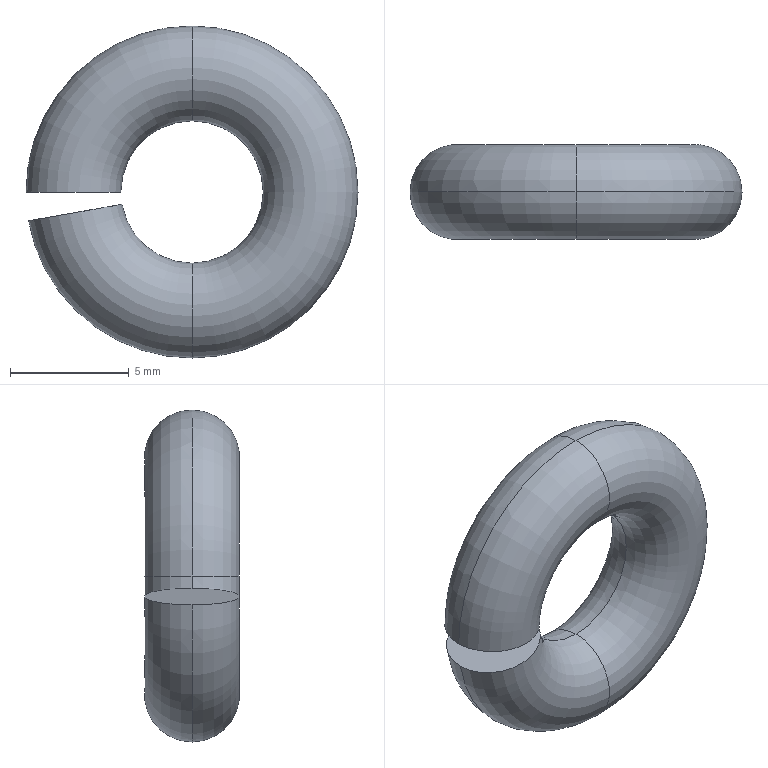Part | SolidWorks | features BaseBody 1 | 1 solid | 8 faces | box 14 x 4 x 14 mm | volume 383.818 mm3 | torus 6 | plane 2
STEP:
#1=CARTESIAN_POINT('',(0.,0.,-7.));
#2=VERTEX_POINT('',#1);
#3=CARTESIAN_POINT('',(0.,0.,-3.));
#4=VERTEX_POINT('',#3);
#5=CARTESIAN_POINT('',(0.,0.,-5.));
#6=DIRECTION('',(1.,0.,0.));
#7=DIRECTION('',(0.,0.,-1.));
#8=AXIS2_PLACEMENT_3D('',#5,#6,#7);
#9=CIRCLE('',#8,2.);
#10=EDGE_CURVE('',#2,#4,#9,.T.);
#11=ORIENTED_EDGE('',*,*,#10,.F.);
#12=CARTESIAN_POINT('',(-6.894,0.,-1.216));
#13=VERTEX_POINT('',#12);
#14=CARTESIAN_POINT('',(0.,0.,0.));
#15=DIRECTION('',(0.,1.,0.));
#16=DIRECTION('',(0.,0.,1.));
#17=AXIS2_PLACEMENT_3D('',#14,#15,#16);
#18=CIRCLE('',#17,7.);
#19=EDGE_CURVE('',#2,#13,#18,.T.);
#20=ORIENTED_EDGE('',*,*,#19,.T.);
#21=CARTESIAN_POINT('',(-2.954,0.,-0.5209));
#22=VERTEX_POINT('',#21);
#23=CARTESIAN_POINT('',(-4.924,0.,-0.8682));
#24=DIRECTION('',(-0.1736,0.,0.9848));
#25=DIRECTION('',(-0.9848,0.,-0.1736));
#26=AXIS2_PLACEMENT_3D('',#23,#24,#25);
#27=CIRCLE('',#26,2.);
#28=EDGE_CURVE('',#22,#13,#27,.T.);
#29=ORIENTED_EDGE('',*,*,#28,.F.);
#30=CARTESIAN_POINT('',(0.,0.,0.));
#31=DIRECTION('',(0.,1.,0.));
#32=DIRECTION('',(0.,0.,1.));
#33=AXIS2_PLACEMENT_3D('',#30,#31,#32);
#34=CIRCLE('',#33,3.);
#35=EDGE_CURVE('',#4,#22,#34,.T.);
#36=ORIENTED_EDGE('',*,*,#35,.F.);
#37=EDGE_LOOP('',(#11,#20,#29,#36));
#38=FACE_OUTER_BOUND('',#37,.T.);
#39=CARTESIAN_POINT('',(0.,0.,0.));
#40=DIRECTION('',(0.,1.,0.));
#41=DIRECTION('',(0.,0.,1.));
#42=AXIS2_PLACEMENT_3D('',#39,#40,#41);
#43=TOROIDAL_SURFACE('',#42,5.,2.);
#44=ADVANCED_FACE('',(#38),#43,.T.);
#45=CARTESIAN_POINT('',(-7.,0.,0.));
#46=VERTEX_POINT('',#45);
#47=CARTESIAN_POINT('',(-3.,0.,0.));
#48=VERTEX_POINT('',#47);
#49=CARTESIAN_POINT('',(-5.,0.,0.));
#50=DIRECTION('',(0.,0.,-1.));
#51=DIRECTION('',(-1.,0.,0.));
#52=AXIS2_PLACEMENT_3D('',#49,#50,#51);
#53=CIRCLE('',#52,2.);
#54=EDGE_CURVE('',#46,#48,#53,.T.);
#55=ORIENTED_EDGE('',*,*,#54,.F.);
#56=CARTESIAN_POINT('',(0.,0.,7.));
#57=VERTEX_POINT('',#56);
#58=CARTESIAN_POINT('',(0.,0.,0.));
#59=DIRECTION('',(0.,1.,0.));
#60=DIRECTION('',(0.,0.,1.));
#61=AXIS2_PLACEMENT_3D('',#58,#59,#60);
#62=CIRCLE('',#61,7.);
#63=EDGE_CURVE('',#46,#57,#62,.T.);
#64=ORIENTED_EDGE('',*,*,#63,.T.);
#65=CARTESIAN_POINT('',(0.,0.,3.));
#66=VERTEX_POINT('',#65);
#67=CARTESIAN_POINT('',(0.,0.,5.));
#68=DIRECTION('',(-1.,0.,0.));
#69=DIRECTION('',(0.,0.,1.));
#70=AXIS2_PLACEMENT_3D('',#67,#68,#69);
#71=CIRCLE('',#70,2.);
#72=EDGE_CURVE('',#57,#66,#71,.T.);
#73=ORIENTED_EDGE('',*,*,#72,.T.);
#74=CARTESIAN_POINT('',(0.,0.,0.));
#75=DIRECTION('',(0.,1.,0.));
#76=DIRECTION('',(0.,0.,1.));
#77=AXIS2_PLACEMENT_3D('',#74,#75,#76);
#78=CIRCLE('',#77,3.);
#79=EDGE_CURVE('',#48,#66,#78,.T.);
#80=ORIENTED_EDGE('',*,*,#79,.F.);
#81=EDGE_LOOP('',(#55,#64,#73,#80));
#82=FACE_OUTER_BOUND('',#81,.T.);
#83=CARTESIAN_POINT('',(0.,0.,0.));
#84=DIRECTION('',(0.,1.,0.));
#85=DIRECTION('',(0.,0.,1.));
#86=AXIS2_PLACEMENT_3D('',#83,#84,#85);
#87=TOROIDAL_SURFACE('',#86,5.,2.);
#88=ADVANCED_FACE('',(#82),#87,.T.);
#89=ORIENTED_EDGE('',*,*,#72,.F.);
#90=CARTESIAN_POINT('',(0.,0.,0.));
#91=DIRECTION('',(0.,1.,0.));
#92=DIRECTION('',(0.,0.,1.));
#93=AXIS2_PLACEMENT_3D('',#90,#91,#92);
#94=CIRCLE('',#93,7.);
#95=EDGE_CURVE('',#57,#2,#94,.T.);
#96=ORIENTED_EDGE('',*,*,#95,.T.);
#97=ORIENTED_EDGE('',*,*,#10,.T.);
#98=CARTESIAN_POINT('',(0.,0.,0.));
#99=DIRECTION('',(0.,1.,0.));
#100=DIRECTION('',(0.,0.,1.));
#101=AXIS2_PLACEMENT_3D('',#98,#99,#100);
#102=CIRCLE('',#101,3.);
#103=EDGE_CURVE('',#66,#4,#102,.T.);
#104=ORIENTED_EDGE('',*,*,#103,.F.);
#105=EDGE_LOOP('',(#89,#96,#97,#104));
#106=FACE_OUTER_BOUND('',#105,.T.);
#107=CARTESIAN_POINT('',(0.,0.,0.));
#108=DIRECTION('',(0.,1.,0.));
#109=DIRECTION('',(0.,0.,1.));
#110=AXIS2_PLACEMENT_3D('',#107,#108,#109);
#111=TOROIDAL_SURFACE('',#110,5.,2.);
#112=ADVANCED_FACE('',(#106),#111,.T.);
#113=ORIENTED_EDGE('',*,*,#95,.F.);
#114=CARTESIAN_POINT('',(0.,0.,5.));
#115=DIRECTION('',(-1.,0.,0.));
#116=DIRECTION('',(0.,0.,1.));
#117=AXIS2_PLACEMENT_3D('',#114,#115,#116);
#118=CIRCLE('',#117,2.);
#119=EDGE_CURVE('',#66,#57,#118,.T.);
#120=ORIENTED_EDGE('',*,*,#119,.F.);
#121=ORIENTED_EDGE('',*,*,#103,.T.);
#122=CARTESIAN_POINT('',(0.,0.,-5.));
#123=DIRECTION('',(1.,0.,0.));
#124=DIRECTION('',(0.,0.,-1.));
#125=AXIS2_PLACEMENT_3D('',#122,#123,#124);
#126=CIRCLE('',#125,2.);
#127=EDGE_CURVE('',#4,#2,#126,.T.);
#128=ORIENTED_EDGE('',*,*,#127,.T.);
#129=EDGE_LOOP('',(#113,#120,#121,#128));
#130=FACE_OUTER_BOUND('',#129,.T.);
#131=CARTESIAN_POINT('',(0.,0.,0.));
#132=DIRECTION('',(0.,1.,0.));
#133=DIRECTION('',(0.,0.,1.));
#134=AXIS2_PLACEMENT_3D('',#131,#132,#133);
#135=TOROIDAL_SURFACE('',#134,5.,2.);
#136=ADVANCED_FACE('',(#130),#135,.T.);
#137=ORIENTED_EDGE('',*,*,#63,.F.);
#138=CARTESIAN_POINT('',(-5.,0.,0.));
#139=DIRECTION('',(0.,0.,-1.));
#140=DIRECTION('',(-1.,0.,0.));
#141=AXIS2_PLACEMENT_3D('',#138,#139,#140);
#142=CIRCLE('',#141,2.);
#143=EDGE_CURVE('',#48,#46,#142,.T.);
#144=ORIENTED_EDGE('',*,*,#143,.F.);
#145=ORIENTED_EDGE('',*,*,#79,.T.);
#146=ORIENTED_EDGE('',*,*,#119,.T.);
#147=EDGE_LOOP('',(#137,#144,#145,#146));
#148=FACE_OUTER_BOUND('',#147,.T.);
#149=CARTESIAN_POINT('',(0.,0.,0.));
#150=DIRECTION('',(0.,1.,0.));
#151=DIRECTION('',(0.,0.,1.));
#152=AXIS2_PLACEMENT_3D('',#149,#150,#151);
#153=TOROIDAL_SURFACE('',#152,5.,2.);
#154=ADVANCED_FACE('',(#148),#153,.T.);
#155=ORIENTED_EDGE('',*,*,#143,.T.);
#156=ORIENTED_EDGE('',*,*,#54,.T.);
#157=EDGE_LOOP('',(#155,#156));
#158=FACE_OUTER_BOUND('',#157,.T.);
#159=CARTESIAN_POINT('',(-5.,0.,0.));
#160=DIRECTION('',(0.,0.,1.));
#161=DIRECTION('',(1.,0.,0.));
#162=AXIS2_PLACEMENT_3D('',#159,#160,#161);
#163=PLANE('',#162);
#164=ADVANCED_FACE('',(#158),#163,.F.);
#165=ORIENTED_EDGE('',*,*,#28,.T.);
#166=CARTESIAN_POINT('',(-4.924,0.,-0.8682));
#167=DIRECTION('',(-0.1736,0.,0.9848));
#168=DIRECTION('',(-0.9848,0.,-0.1736));
#169=AXIS2_PLACEMENT_3D('',#166,#167,#168);
#170=CIRCLE('',#169,2.);
#171=EDGE_CURVE('',#13,#22,#170,.T.);
#172=ORIENTED_EDGE('',*,*,#171,.T.);
#173=EDGE_LOOP('',(#165,#172));
#174=FACE_OUTER_BOUND('',#173,.T.);
#175=CARTESIAN_POINT('',(-4.924,0.,-0.8682));
#176=DIRECTION('',(-0.1736,0.,0.9848));
#177=DIRECTION('',(0.,1.,0.));
#178=AXIS2_PLACEMENT_3D('',#175,#176,#177);
#179=PLANE('',#178);
#180=ADVANCED_FACE('',(#174),#179,.T.);
#181=ORIENTED_EDGE('',*,*,#19,.F.);
#182=ORIENTED_EDGE('',*,*,#127,.F.);
#183=ORIENTED_EDGE('',*,*,#35,.T.);
#184=ORIENTED_EDGE('',*,*,#171,.F.);
#185=EDGE_LOOP('',(#181,#182,#183,#184));
#186=FACE_OUTER_BOUND('',#185,.T.);
#187=CARTESIAN_POINT('',(0.,0.,0.));
#188=DIRECTION('',(0.,1.,0.));
#189=DIRECTION('',(0.,0.,1.));
#190=AXIS2_PLACEMENT_3D('',#187,#188,#189);
#191=TOROIDAL_SURFACE('',#190,5.,2.);
#192=ADVANCED_FACE('',(#186),#191,.T.);
#193=CLOSED_SHELL('',(#44,#88,#112,#136,#154,#164,#180,#192));
#194=MANIFOLD_SOLID_BREP('',#193);
#195=CARTESIAN_POINT('',(0.,0.,0.));
#196=DIRECTION('',(0.,0.,1.));
#197=DIRECTION('',(1.,0.,0.));
#198=AXIS2_PLACEMENT_3D('',#195,#196,#197);
#199=(LENGTH_UNIT()NAMED_UNIT(*)SI_UNIT(.MILLI.,.METRE.));
#200=UNCERTAINTY_MEASURE_WITH_UNIT(LENGTH_MEASURE(0.00001),#199,'','');
#201=(NAMED_UNIT(*)PLANE_ANGLE_UNIT()SI_UNIT($,.RADIAN.));
#202=(NAMED_UNIT(*)SI_UNIT($,.STERADIAN.)SOLID_ANGLE_UNIT());
#203=(GEOMETRIC_REPRESENTATION_CONTEXT(3)GLOBAL_UNCERTAINTY_ASSIGNED_CONTEXT((#200))GLOBAL_UNIT_ASSIGNED_CONTEXT((#199,#201,#202))REPRESENTATION_CONTEXT('',''));
#204=ADVANCED_BREP_SHAPE_REPRESENTATION('',(#194,#198),#203);